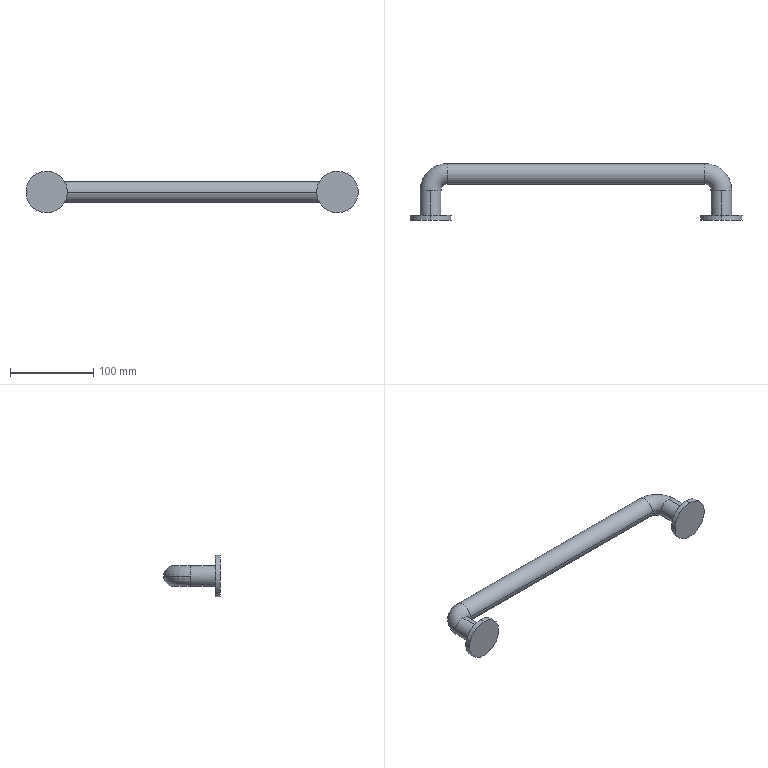Part | SolidWorks | features BaseBody 1 | 1 solid | 18 faces | box 400 x 68.5 x 50 mm | volume 236028 mm3 | cylinder 10 | plane 4 | torus 4 | commonest cylinder face diameters 25 x6 50 x4
STEP:
#1=CARTESIAN_POINT('',(175.,0.,-12.5));
#2=VERTEX_POINT('',#1);
#3=CARTESIAN_POINT('',(175.,0.,12.5));
#4=VERTEX_POINT('',#3);
#5=CARTESIAN_POINT('',(175.,0.,0.));
#6=DIRECTION('',(0.,-1.,0.));
#7=DIRECTION('',(0.,0.,1.));
#8=AXIS2_PLACEMENT_3D('',#5,#6,#7);
#9=CIRCLE('',#8,12.5);
#10=EDGE_CURVE('',#2,#4,#9,.T.);
#11=ORIENTED_EDGE('',*,*,#10,.T.);
#12=CARTESIAN_POINT('',(175.,0.,0.));
#13=DIRECTION('',(0.,-1.,0.));
#14=DIRECTION('',(0.,0.,1.));
#15=AXIS2_PLACEMENT_3D('',#12,#13,#14);
#16=CIRCLE('',#15,12.5);
#17=EDGE_CURVE('',#4,#2,#16,.T.);
#18=ORIENTED_EDGE('',*,*,#17,.T.);
#19=EDGE_LOOP('',(#11,#18));
#20=FACE_BOUND('',#19,.T.);
#21=CARTESIAN_POINT('',(175.,0.,25.));
#22=VERTEX_POINT('',#21);
#23=CARTESIAN_POINT('',(175.,0.,-25.));
#24=VERTEX_POINT('',#23);
#25=CARTESIAN_POINT('',(175.,0.,0.));
#26=DIRECTION('',(0.,-1.,0.));
#27=DIRECTION('',(0.,0.,-1.));
#28=AXIS2_PLACEMENT_3D('',#25,#26,#27);
#29=CIRCLE('',#28,25.);
#30=EDGE_CURVE('',#22,#24,#29,.T.);
#31=ORIENTED_EDGE('',*,*,#30,.F.);
#32=CARTESIAN_POINT('',(175.,0.,0.));
#33=DIRECTION('',(0.,-1.,0.));
#34=DIRECTION('',(0.,0.,-1.));
#35=AXIS2_PLACEMENT_3D('',#32,#33,#34);
#36=CIRCLE('',#35,25.);
#37=EDGE_CURVE('',#24,#22,#36,.T.);
#38=ORIENTED_EDGE('',*,*,#37,.F.);
#39=EDGE_LOOP('',(#31,#38));
#40=FACE_OUTER_BOUND('',#39,.T.);
#41=CARTESIAN_POINT('',(175.,0.,0.));
#42=DIRECTION('',(0.,-1.,0.));
#43=DIRECTION('',(0.,0.,-1.));
#44=AXIS2_PLACEMENT_3D('',#41,#42,#43);
#45=PLANE('',#44);
#46=ADVANCED_FACE('',(#20,#40),#45,.F.);
#47=CARTESIAN_POINT('',(175.,-6.,25.));
#48=VERTEX_POINT('',#47);
#49=CARTESIAN_POINT('',(175.,-6.,-25.));
#50=VERTEX_POINT('',#49);
#51=CARTESIAN_POINT('',(175.,-6.,0.));
#52=DIRECTION('',(0.,-1.,0.));
#53=DIRECTION('',(0.,0.,-1.));
#54=AXIS2_PLACEMENT_3D('',#51,#52,#53);
#55=CIRCLE('',#54,25.);
#56=EDGE_CURVE('',#48,#50,#55,.T.);
#57=ORIENTED_EDGE('',*,*,#56,.T.);
#58=CARTESIAN_POINT('',(175.,-6.,0.));
#59=DIRECTION('',(0.,-1.,0.));
#60=DIRECTION('',(0.,0.,-1.));
#61=AXIS2_PLACEMENT_3D('',#58,#59,#60);
#62=CIRCLE('',#61,25.);
#63=EDGE_CURVE('',#50,#48,#62,.T.);
#64=ORIENTED_EDGE('',*,*,#63,.T.);
#65=EDGE_LOOP('',(#57,#64));
#66=FACE_OUTER_BOUND('',#65,.T.);
#67=CARTESIAN_POINT('',(175.,-6.,0.));
#68=DIRECTION('',(0.,-1.,0.));
#69=DIRECTION('',(0.,0.,-1.));
#70=AXIS2_PLACEMENT_3D('',#67,#68,#69);
#71=PLANE('',#70);
#72=ADVANCED_FACE('',(#66),#71,.T.);
#73=CARTESIAN_POINT('',(175.,-6.,-25.));
#74=DIRECTION('',(0.,1.,0.));
#75=VECTOR('',#74,1000.);
#76=LINE('',#73,#75);
#77=EDGE_CURVE('',#50,#24,#76,.T.);
#78=ORIENTED_EDGE('',*,*,#77,.F.);
#79=ORIENTED_EDGE('',*,*,#56,.F.);
#80=CARTESIAN_POINT('',(175.,-6.,25.));
#81=DIRECTION('',(0.,1.,0.));
#82=VECTOR('',#81,1000.);
#83=LINE('',#80,#82);
#84=EDGE_CURVE('',#48,#22,#83,.T.);
#85=ORIENTED_EDGE('',*,*,#84,.T.);
#86=ORIENTED_EDGE('',*,*,#30,.T.);
#87=EDGE_LOOP('',(#78,#79,#85,#86));
#88=FACE_OUTER_BOUND('',#87,.T.);
#89=CARTESIAN_POINT('',(175.,-6.,0.));
#90=DIRECTION('',(0.,1.,0.));
#91=DIRECTION('',(0.,0.,1.));
#92=AXIS2_PLACEMENT_3D('',#89,#90,#91);
#93=CYLINDRICAL_SURFACE('',#92,25.);
#94=ADVANCED_FACE('',(#88),#93,.T.);
#95=CARTESIAN_POINT('',(-175.,0.,12.5));
#96=VERTEX_POINT('',#95);
#97=CARTESIAN_POINT('',(-175.,0.,-12.5));
#98=VERTEX_POINT('',#97);
#99=CARTESIAN_POINT('',(-175.,0.,0.));
#100=DIRECTION('',(0.,1.,0.));
#101=DIRECTION('',(0.,0.,1.));
#102=AXIS2_PLACEMENT_3D('',#99,#100,#101);
#103=CIRCLE('',#102,12.5);
#104=EDGE_CURVE('',#96,#98,#103,.T.);
#105=ORIENTED_EDGE('',*,*,#104,.F.);
#106=CARTESIAN_POINT('',(-175.,0.,0.));
#107=DIRECTION('',(0.,1.,0.));
#108=DIRECTION('',(0.,0.,1.));
#109=AXIS2_PLACEMENT_3D('',#106,#107,#108);
#110=CIRCLE('',#109,12.5);
#111=EDGE_CURVE('',#98,#96,#110,.T.);
#112=ORIENTED_EDGE('',*,*,#111,.F.);
#113=EDGE_LOOP('',(#105,#112));
#114=FACE_BOUND('',#113,.T.);
#115=CARTESIAN_POINT('',(-175.,0.,25.));
#116=VERTEX_POINT('',#115);
#117=CARTESIAN_POINT('',(-175.,0.,-25.));
#118=VERTEX_POINT('',#117);
#119=CARTESIAN_POINT('',(-175.,0.,0.));
#120=DIRECTION('',(0.,-1.,0.));
#121=DIRECTION('',(0.,0.,-1.));
#122=AXIS2_PLACEMENT_3D('',#119,#120,#121);
#123=CIRCLE('',#122,25.);
#124=EDGE_CURVE('',#116,#118,#123,.T.);
#125=ORIENTED_EDGE('',*,*,#124,.F.);
#126=CARTESIAN_POINT('',(-175.,0.,0.));
#127=DIRECTION('',(0.,-1.,0.));
#128=DIRECTION('',(0.,0.,-1.));
#129=AXIS2_PLACEMENT_3D('',#126,#127,#128);
#130=CIRCLE('',#129,25.);
#131=EDGE_CURVE('',#118,#116,#130,.T.);
#132=ORIENTED_EDGE('',*,*,#131,.F.);
#133=EDGE_LOOP('',(#125,#132));
#134=FACE_OUTER_BOUND('',#133,.T.);
#135=CARTESIAN_POINT('',(-175.,0.,0.));
#136=DIRECTION('',(0.,-1.,0.));
#137=DIRECTION('',(0.,0.,-1.));
#138=AXIS2_PLACEMENT_3D('',#135,#136,#137);
#139=PLANE('',#138);
#140=ADVANCED_FACE('',(#114,#134),#139,.F.);
#141=CARTESIAN_POINT('',(-175.,-6.,25.));
#142=VERTEX_POINT('',#141);
#143=CARTESIAN_POINT('',(-175.,-6.,-25.));
#144=VERTEX_POINT('',#143);
#145=CARTESIAN_POINT('',(-175.,-6.,0.));
#146=DIRECTION('',(0.,-1.,0.));
#147=DIRECTION('',(0.,0.,-1.));
#148=AXIS2_PLACEMENT_3D('',#145,#146,#147);
#149=CIRCLE('',#148,25.);
#150=EDGE_CURVE('',#142,#144,#149,.T.);
#151=ORIENTED_EDGE('',*,*,#150,.T.);
#152=CARTESIAN_POINT('',(-175.,-6.,0.));
#153=DIRECTION('',(0.,-1.,0.));
#154=DIRECTION('',(0.,0.,-1.));
#155=AXIS2_PLACEMENT_3D('',#152,#153,#154);
#156=CIRCLE('',#155,25.);
#157=EDGE_CURVE('',#144,#142,#156,.T.);
#158=ORIENTED_EDGE('',*,*,#157,.T.);
#159=EDGE_LOOP('',(#151,#158));
#160=FACE_OUTER_BOUND('',#159,.T.);
#161=CARTESIAN_POINT('',(-175.,-6.,0.));
#162=DIRECTION('',(0.,-1.,0.));
#163=DIRECTION('',(0.,0.,-1.));
#164=AXIS2_PLACEMENT_3D('',#161,#162,#163);
#165=PLANE('',#164);
#166=ADVANCED_FACE('',(#160),#165,.T.);
#167=CARTESIAN_POINT('',(-175.,-6.,-25.));
#168=DIRECTION('',(0.,1.,0.));
#169=VECTOR('',#168,1000.);
#170=LINE('',#167,#169);
#171=EDGE_CURVE('',#144,#118,#170,.T.);
#172=ORIENTED_EDGE('',*,*,#171,.F.);
#173=ORIENTED_EDGE('',*,*,#150,.F.);
#174=CARTESIAN_POINT('',(-175.,-6.,25.));
#175=DIRECTION('',(0.,1.,0.));
#176=VECTOR('',#175,1000.);
#177=LINE('',#174,#176);
#178=EDGE_CURVE('',#142,#116,#177,.T.);
#179=ORIENTED_EDGE('',*,*,#178,.T.);
#180=ORIENTED_EDGE('',*,*,#124,.T.);
#181=EDGE_LOOP('',(#172,#173,#179,#180));
#182=FACE_OUTER_BOUND('',#181,.T.);
#183=CARTESIAN_POINT('',(-175.,-6.,0.));
#184=DIRECTION('',(0.,1.,0.));
#185=DIRECTION('',(0.,0.,1.));
#186=AXIS2_PLACEMENT_3D('',#183,#184,#185);
#187=CYLINDRICAL_SURFACE('',#186,25.);
#188=ADVANCED_FACE('',(#182),#187,.T.);
#189=CARTESIAN_POINT('',(-175.,30.,-12.5));
#190=VERTEX_POINT('',#189);
#191=CARTESIAN_POINT('',(-175.,0.,-12.5));
#192=DIRECTION('',(0.,1.,0.));
#193=VECTOR('',#192,1000.);
#194=LINE('',#191,#193);
#195=EDGE_CURVE('',#98,#190,#194,.T.);
#196=ORIENTED_EDGE('',*,*,#195,.F.);
#197=ORIENTED_EDGE('',*,*,#111,.T.);
#198=CARTESIAN_POINT('',(-175.,30.,12.5));
#199=VERTEX_POINT('',#198);
#200=CARTESIAN_POINT('',(-175.,0.,12.5));
#201=DIRECTION('',(0.,1.,0.));
#202=VECTOR('',#201,1000.);
#203=LINE('',#200,#202);
#204=EDGE_CURVE('',#96,#199,#203,.T.);
#205=ORIENTED_EDGE('',*,*,#204,.T.);
#206=CARTESIAN_POINT('',(-187.5,30.,0.));
#207=VERTEX_POINT('',#206);
#208=CARTESIAN_POINT('',(-175.,30.,0.));
#209=DIRECTION('',(0.,1.,0.));
#210=DIRECTION('',(0.,0.,1.));
#211=AXIS2_PLACEMENT_3D('',#208,#209,#210);
#212=CIRCLE('',#211,12.5);
#213=EDGE_CURVE('',#207,#199,#212,.T.);
#214=ORIENTED_EDGE('',*,*,#213,.F.);
#215=CARTESIAN_POINT('',(-175.,30.,0.));
#216=DIRECTION('',(0.,1.,0.));
#217=DIRECTION('',(0.,0.,1.));
#218=AXIS2_PLACEMENT_3D('',#215,#216,#217);
#219=CIRCLE('',#218,12.5);
#220=EDGE_CURVE('',#190,#207,#219,.T.);
#221=ORIENTED_EDGE('',*,*,#220,.F.);
#222=EDGE_LOOP('',(#196,#197,#205,#214,#221));
#223=FACE_OUTER_BOUND('',#222,.T.);
#224=CARTESIAN_POINT('',(-175.,0.,0.));
#225=DIRECTION('',(0.,1.,0.));
#226=DIRECTION('',(0.,0.,1.));
#227=AXIS2_PLACEMENT_3D('',#224,#225,#226);
#228=CYLINDRICAL_SURFACE('',#227,12.5);
#229=ADVANCED_FACE('',(#223),#228,.T.);
#230=CARTESIAN_POINT('',(-155.,62.5,0.));
#231=VERTEX_POINT('',#230);
#232=CARTESIAN_POINT('',(-155.,30.,0.));
#233=DIRECTION('',(0.,0.,-1.));
#234=DIRECTION('',(-1.,0.,0.));
#235=AXIS2_PLACEMENT_3D('',#232,#233,#234);
#236=CIRCLE('',#235,32.5);
#237=EDGE_CURVE('',#207,#231,#236,.T.);
#238=ORIENTED_EDGE('',*,*,#237,.F.);
#239=ORIENTED_EDGE('',*,*,#213,.T.);
#240=CARTESIAN_POINT('',(-162.5,30.,0.));
#241=VERTEX_POINT('',#240);
#242=CARTESIAN_POINT('',(-175.,30.,0.));
#243=DIRECTION('',(0.,1.,0.));
#244=DIRECTION('',(0.,0.,1.));
#245=AXIS2_PLACEMENT_3D('',#242,#243,#244);
#246=CIRCLE('',#245,12.5);
#247=EDGE_CURVE('',#199,#241,#246,.T.);
#248=ORIENTED_EDGE('',*,*,#247,.T.);
#249=CARTESIAN_POINT('',(-155.,37.5,0.));
#250=VERTEX_POINT('',#249);
#251=CARTESIAN_POINT('',(-155.,30.,0.));
#252=DIRECTION('',(0.,0.,-1.));
#253=DIRECTION('',(-1.,0.,0.));
#254=AXIS2_PLACEMENT_3D('',#251,#252,#253);
#255=CIRCLE('',#254,7.5);
#256=EDGE_CURVE('',#241,#250,#255,.T.);
#257=ORIENTED_EDGE('',*,*,#256,.T.);
#258=CARTESIAN_POINT('',(-155.,50.,0.));
#259=DIRECTION('',(1.,0.,0.));
#260=DIRECTION('',(0.,0.,1.));
#261=AXIS2_PLACEMENT_3D('',#258,#259,#260);
#262=CIRCLE('',#261,12.5);
#263=EDGE_CURVE('',#231,#250,#262,.T.);
#264=ORIENTED_EDGE('',*,*,#263,.F.);
#265=EDGE_LOOP('',(#238,#239,#248,#257,#264));
#266=FACE_OUTER_BOUND('',#265,.T.);
#267=CARTESIAN_POINT('',(-155.,30.,0.));
#268=DIRECTION('',(0.,0.,-1.));
#269=DIRECTION('',(-1.,0.,0.));
#270=AXIS2_PLACEMENT_3D('',#267,#268,#269);
#271=TOROIDAL_SURFACE('',#270,20.,12.5);
#272=ADVANCED_FACE('',(#266),#271,.T.);
#273=CARTESIAN_POINT('',(155.,37.5,0.));
#274=VERTEX_POINT('',#273);
#275=CARTESIAN_POINT('',(-155.,37.5,0.));
#276=DIRECTION('',(1.,0.,0.));
#277=VECTOR('',#276,1000.);
#278=LINE('',#275,#277);
#279=EDGE_CURVE('',#250,#274,#278,.T.);
#280=ORIENTED_EDGE('',*,*,#279,.F.);
#281=CARTESIAN_POINT('',(-155.,50.,0.));
#282=DIRECTION('',(1.,0.,0.));
#283=DIRECTION('',(0.,0.,1.));
#284=AXIS2_PLACEMENT_3D('',#281,#282,#283);
#285=CIRCLE('',#284,12.5);
#286=EDGE_CURVE('',#250,#231,#285,.T.);
#287=ORIENTED_EDGE('',*,*,#286,.T.);
#288=CARTESIAN_POINT('',(155.,62.5,0.));
#289=VERTEX_POINT('',#288);
#290=CARTESIAN_POINT('',(-155.,62.5,0.));
#291=DIRECTION('',(1.,0.,0.));
#292=VECTOR('',#291,1000.);
#293=LINE('',#290,#292);
#294=EDGE_CURVE('',#231,#289,#293,.T.);
#295=ORIENTED_EDGE('',*,*,#294,.T.);
#296=CARTESIAN_POINT('',(155.,50.,0.));
#297=DIRECTION('',(1.,0.,0.));
#298=DIRECTION('',(0.,0.,1.));
#299=AXIS2_PLACEMENT_3D('',#296,#297,#298);
#300=CIRCLE('',#299,12.5);
#301=EDGE_CURVE('',#274,#289,#300,.T.);
#302=ORIENTED_EDGE('',*,*,#301,.F.);
#303=EDGE_LOOP('',(#280,#287,#295,#302));
#304=FACE_OUTER_BOUND('',#303,.T.);
#305=CARTESIAN_POINT('',(-155.,50.,0.));
#306=DIRECTION('',(1.,0.,0.));
#307=DIRECTION('',(0.,1.,0.));
#308=AXIS2_PLACEMENT_3D('',#305,#306,#307);
#309=CYLINDRICAL_SURFACE('',#308,12.5);
#310=ADVANCED_FACE('',(#304),#309,.T.);
#311=CARTESIAN_POINT('',(187.5,30.,0.));
#312=VERTEX_POINT('',#311);
#313=CARTESIAN_POINT('',(155.,30.,0.));
#314=DIRECTION('',(0.,0.,-1.));
#315=DIRECTION('',(-1.,0.,0.));
#316=AXIS2_PLACEMENT_3D('',#313,#314,#315);
#317=CIRCLE('',#316,32.5);
#318=EDGE_CURVE('',#289,#312,#317,.T.);
#319=ORIENTED_EDGE('',*,*,#318,.F.);
#320=CARTESIAN_POINT('',(155.,50.,0.));
#321=DIRECTION('',(1.,0.,0.));
#322=DIRECTION('',(0.,0.,1.));
#323=AXIS2_PLACEMENT_3D('',#320,#321,#322);
#324=CIRCLE('',#323,12.5);
#325=EDGE_CURVE('',#289,#274,#324,.T.);
#326=ORIENTED_EDGE('',*,*,#325,.T.);
#327=CARTESIAN_POINT('',(162.5,30.,0.));
#328=VERTEX_POINT('',#327);
#329=CARTESIAN_POINT('',(155.,30.,0.));
#330=DIRECTION('',(0.,0.,-1.));
#331=DIRECTION('',(-1.,0.,0.));
#332=AXIS2_PLACEMENT_3D('',#329,#330,#331);
#333=CIRCLE('',#332,7.5);
#334=EDGE_CURVE('',#274,#328,#333,.T.);
#335=ORIENTED_EDGE('',*,*,#334,.T.);
#336=CARTESIAN_POINT('',(175.,30.,12.5));
#337=VERTEX_POINT('',#336);
#338=CARTESIAN_POINT('',(175.,30.,0.));
#339=DIRECTION('',(0.,-1.,0.));
#340=DIRECTION('',(0.,0.,1.));
#341=AXIS2_PLACEMENT_3D('',#338,#339,#340);
#342=CIRCLE('',#341,12.5);
#343=EDGE_CURVE('',#337,#328,#342,.T.);
#344=ORIENTED_EDGE('',*,*,#343,.F.);
#345=CARTESIAN_POINT('',(175.,30.,0.));
#346=DIRECTION('',(0.,-1.,0.));
#347=DIRECTION('',(0.,0.,1.));
#348=AXIS2_PLACEMENT_3D('',#345,#346,#347);
#349=CIRCLE('',#348,12.5);
#350=EDGE_CURVE('',#312,#337,#349,.T.);
#351=ORIENTED_EDGE('',*,*,#350,.F.);
#352=EDGE_LOOP('',(#319,#326,#335,#344,#351));
#353=FACE_OUTER_BOUND('',#352,.T.);
#354=CARTESIAN_POINT('',(155.,30.,0.));
#355=DIRECTION('',(0.,0.,-1.));
#356=DIRECTION('',(-1.,0.,0.));
#357=AXIS2_PLACEMENT_3D('',#354,#355,#356);
#358=TOROIDAL_SURFACE('',#357,20.,12.5);
#359=ADVANCED_FACE('',(#353),#358,.T.);
#360=CARTESIAN_POINT('',(175.,30.,12.5));
#361=DIRECTION('',(0.,-1.,0.));
#362=VECTOR('',#361,1000.);
#363=LINE('',#360,#362);
#364=EDGE_CURVE('',#337,#4,#363,.T.);
#365=ORIENTED_EDGE('',*,*,#364,.F.);
#366=ORIENTED_EDGE('',*,*,#343,.T.);
#367=CARTESIAN_POINT('',(175.,30.,-12.5));
#368=VERTEX_POINT('',#367);
#369=CARTESIAN_POINT('',(175.,30.,0.));
#370=DIRECTION('',(0.,-1.,0.));
#371=DIRECTION('',(0.,0.,1.));
#372=AXIS2_PLACEMENT_3D('',#369,#370,#371);
#373=CIRCLE('',#372,12.5);
#374=EDGE_CURVE('',#328,#368,#373,.T.);
#375=ORIENTED_EDGE('',*,*,#374,.T.);
#376=CARTESIAN_POINT('',(175.,30.,-12.5));
#377=DIRECTION('',(0.,-1.,0.));
#378=VECTOR('',#377,1000.);
#379=LINE('',#376,#378);
#380=EDGE_CURVE('',#368,#2,#379,.T.);
#381=ORIENTED_EDGE('',*,*,#380,.T.);
#382=ORIENTED_EDGE('',*,*,#17,.F.);
#383=EDGE_LOOP('',(#365,#366,#375,#381,#382));
#384=FACE_OUTER_BOUND('',#383,.T.);
#385=CARTESIAN_POINT('',(175.,30.,0.));
#386=DIRECTION('',(0.,-1.,0.));
#387=DIRECTION('',(0.,0.,-1.));
#388=AXIS2_PLACEMENT_3D('',#385,#386,#387);
#389=CYLINDRICAL_SURFACE('',#388,12.5);
#390=ADVANCED_FACE('',(#384),#389,.T.);
#391=ORIENTED_EDGE('',*,*,#104,.T.);
#392=ORIENTED_EDGE('',*,*,#195,.T.);
#393=CARTESIAN_POINT('',(-175.,30.,0.));
#394=DIRECTION('',(0.,1.,0.));
#395=DIRECTION('',(0.,0.,1.));
#396=AXIS2_PLACEMENT_3D('',#393,#394,#395);
#397=CIRCLE('',#396,12.5);
#398=EDGE_CURVE('',#241,#190,#397,.T.);
#399=ORIENTED_EDGE('',*,*,#398,.F.);
#400=ORIENTED_EDGE('',*,*,#247,.F.);
#401=ORIENTED_EDGE('',*,*,#204,.F.);
#402=EDGE_LOOP('',(#391,#392,#399,#400,#401));
#403=FACE_OUTER_BOUND('',#402,.T.);
#404=CARTESIAN_POINT('',(-175.,0.,0.));
#405=DIRECTION('',(0.,1.,0.));
#406=DIRECTION('',(0.,0.,1.));
#407=AXIS2_PLACEMENT_3D('',#404,#405,#406);
#408=CYLINDRICAL_SURFACE('',#407,12.5);
#409=ADVANCED_FACE('',(#403),#408,.T.);
#410=ORIENTED_EDGE('',*,*,#263,.T.);
#411=ORIENTED_EDGE('',*,*,#279,.T.);
#412=ORIENTED_EDGE('',*,*,#325,.F.);
#413=ORIENTED_EDGE('',*,*,#294,.F.);
#414=EDGE_LOOP('',(#410,#411,#412,#413));
#415=FACE_OUTER_BOUND('',#414,.T.);
#416=CARTESIAN_POINT('',(-155.,50.,0.));
#417=DIRECTION('',(1.,0.,0.));
#418=DIRECTION('',(0.,1.,0.));
#419=AXIS2_PLACEMENT_3D('',#416,#417,#418);
#420=CYLINDRICAL_SURFACE('',#419,12.5);
#421=ADVANCED_FACE('',(#415),#420,.T.);
#422=CARTESIAN_POINT('',(175.,30.,0.));
#423=DIRECTION('',(0.,-1.,0.));
#424=DIRECTION('',(0.,0.,1.));
#425=AXIS2_PLACEMENT_3D('',#422,#423,#424);
#426=CIRCLE('',#425,12.5);
#427=EDGE_CURVE('',#368,#312,#426,.T.);
#428=ORIENTED_EDGE('',*,*,#427,.T.);
#429=ORIENTED_EDGE('',*,*,#350,.T.);
#430=ORIENTED_EDGE('',*,*,#364,.T.);
#431=ORIENTED_EDGE('',*,*,#10,.F.);
#432=ORIENTED_EDGE('',*,*,#380,.F.);
#433=EDGE_LOOP('',(#428,#429,#430,#431,#432));
#434=FACE_OUTER_BOUND('',#433,.T.);
#435=CARTESIAN_POINT('',(175.,30.,0.));
#436=DIRECTION('',(0.,-1.,0.));
#437=DIRECTION('',(0.,0.,-1.));
#438=AXIS2_PLACEMENT_3D('',#435,#436,#437);
#439=CYLINDRICAL_SURFACE('',#438,12.5);
#440=ADVANCED_FACE('',(#434),#439,.T.);
#441=ORIENTED_EDGE('',*,*,#157,.F.);
#442=ORIENTED_EDGE('',*,*,#171,.T.);
#443=ORIENTED_EDGE('',*,*,#131,.T.);
#444=ORIENTED_EDGE('',*,*,#178,.F.);
#445=EDGE_LOOP('',(#441,#442,#443,#444));
#446=FACE_OUTER_BOUND('',#445,.T.);
#447=CARTESIAN_POINT('',(-175.,-6.,0.));
#448=DIRECTION('',(0.,1.,0.));
#449=DIRECTION('',(0.,0.,1.));
#450=AXIS2_PLACEMENT_3D('',#447,#448,#449);
#451=CYLINDRICAL_SURFACE('',#450,25.);
#452=ADVANCED_FACE('',(#446),#451,.T.);
#453=ORIENTED_EDGE('',*,*,#63,.F.);
#454=ORIENTED_EDGE('',*,*,#77,.T.);
#455=ORIENTED_EDGE('',*,*,#37,.T.);
#456=ORIENTED_EDGE('',*,*,#84,.F.);
#457=EDGE_LOOP('',(#453,#454,#455,#456));
#458=FACE_OUTER_BOUND('',#457,.T.);
#459=CARTESIAN_POINT('',(175.,-6.,0.));
#460=DIRECTION('',(0.,1.,0.));
#461=DIRECTION('',(0.,0.,1.));
#462=AXIS2_PLACEMENT_3D('',#459,#460,#461);
#463=CYLINDRICAL_SURFACE('',#462,25.);
#464=ADVANCED_FACE('',(#458),#463,.T.);
#465=ORIENTED_EDGE('',*,*,#220,.T.);
#466=ORIENTED_EDGE('',*,*,#237,.T.);
#467=ORIENTED_EDGE('',*,*,#286,.F.);
#468=ORIENTED_EDGE('',*,*,#256,.F.);
#469=ORIENTED_EDGE('',*,*,#398,.T.);
#470=EDGE_LOOP('',(#465,#466,#467,#468,#469));
#471=FACE_OUTER_BOUND('',#470,.T.);
#472=CARTESIAN_POINT('',(-155.,30.,0.));
#473=DIRECTION('',(0.,0.,-1.));
#474=DIRECTION('',(-1.,0.,0.));
#475=AXIS2_PLACEMENT_3D('',#472,#473,#474);
#476=TOROIDAL_SURFACE('',#475,20.,12.5);
#477=ADVANCED_FACE('',(#471),#476,.T.);
#478=ORIENTED_EDGE('',*,*,#301,.T.);
#479=ORIENTED_EDGE('',*,*,#318,.T.);
#480=ORIENTED_EDGE('',*,*,#427,.F.);
#481=ORIENTED_EDGE('',*,*,#374,.F.);
#482=ORIENTED_EDGE('',*,*,#334,.F.);
#483=EDGE_LOOP('',(#478,#479,#480,#481,#482));
#484=FACE_OUTER_BOUND('',#483,.T.);
#485=CARTESIAN_POINT('',(155.,30.,0.));
#486=DIRECTION('',(0.,0.,-1.));
#487=DIRECTION('',(-1.,0.,0.));
#488=AXIS2_PLACEMENT_3D('',#485,#486,#487);
#489=TOROIDAL_SURFACE('',#488,20.,12.5);
#490=ADVANCED_FACE('',(#484),#489,.T.);
#491=CLOSED_SHELL('',(#46,#72,#94,#140,#166,#188,#229,#272,#310,#359,#390,#409,#421,#440,#452,#464,#477,#490));
#492=MANIFOLD_SOLID_BREP('',#491);
#493=CARTESIAN_POINT('',(0.,0.,0.));
#494=DIRECTION('',(0.,0.,1.));
#495=DIRECTION('',(1.,0.,0.));
#496=AXIS2_PLACEMENT_3D('',#493,#494,#495);
#497=(LENGTH_UNIT()NAMED_UNIT(*)SI_UNIT(.MILLI.,.METRE.));
#498=UNCERTAINTY_MEASURE_WITH_UNIT(LENGTH_MEASURE(0.00001),#497,'','');
#499=(NAMED_UNIT(*)PLANE_ANGLE_UNIT()SI_UNIT($,.RADIAN.));
#500=(NAMED_UNIT(*)SI_UNIT($,.STERADIAN.)SOLID_ANGLE_UNIT());
#501=(GEOMETRIC_REPRESENTATION_CONTEXT(3)GLOBAL_UNCERTAINTY_ASSIGNED_CONTEXT((#498))GLOBAL_UNIT_ASSIGNED_CONTEXT((#497,#499,#500))REPRESENTATION_CONTEXT('',''));
#502=ADVANCED_BREP_SHAPE_REPRESENTATION('',(#492,#496),#501);